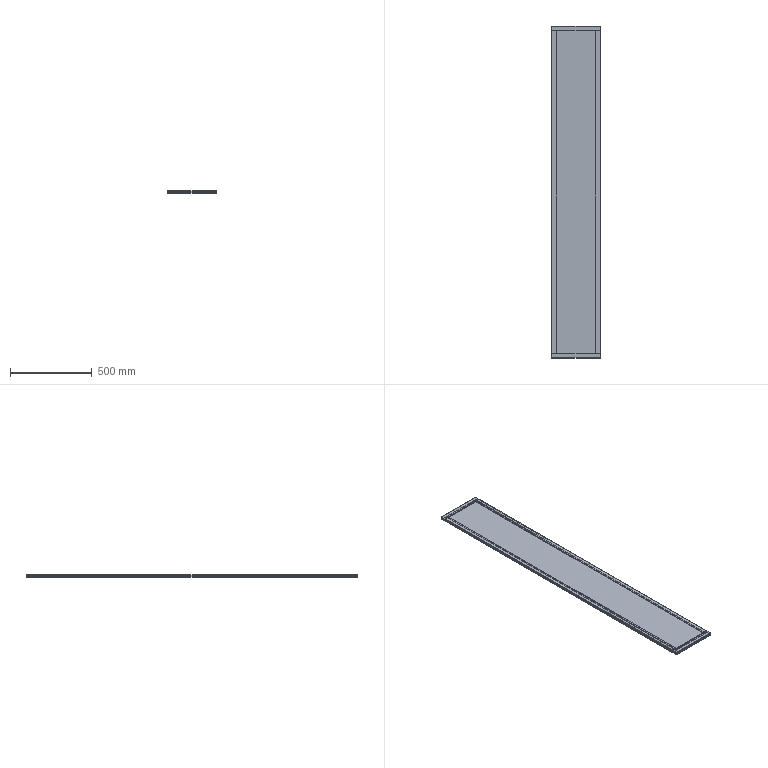Part | 5 solids | 167 faces | box 295 x 2036 x 18 mm | volume 5902072 mm3 | plane 98 | cylinder 69 | commonest cylinder face diameters 1.1 x24 3.6 x20 5.8 x20 1 x5